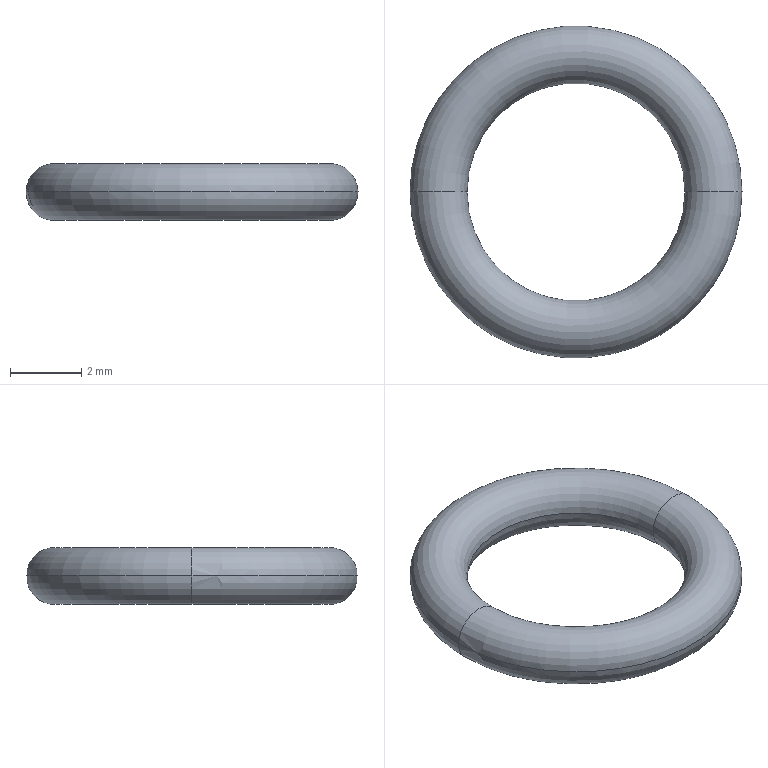Part | STEP file | o-rings_am_J515160x0061H | 1 solid | 4 faces | box 9.3 x 9.3 x 1.6 mm | volume 48.637 mm3 | torus 4
STEP:
#1=CARTESIAN_POINT('',(0.,0.,0.));
#2=DIRECTION('',(0.,0.,1.));
#3=DIRECTION('',(1.,0.,0.));
#4=AXIS2_PLACEMENT_3D('',#1,#2,#3);
#5=CARTESIAN_POINT('',(4.65,0.,0.));
#6=VERTEX_POINT('',#5);
#7=CARTESIAN_POINT('',(3.05,0.,0.));
#8=VERTEX_POINT('',#7);
#9=CARTESIAN_POINT('',(3.85,0.,0.));
#10=DIRECTION('',(0.,1.,0.));
#11=DIRECTION('',(-1.,0.,0.));
#12=AXIS2_PLACEMENT_3D('',#9,#10,#11);
#13=CIRCLE('',#12,0.8);
#14=CARTESIAN_POINT('',(0.,0.,0.));
#15=DIRECTION('',(0.,0.,-1.));
#16=DIRECTION('',(-1.,0.,0.));
#17=AXIS2_PLACEMENT_3D('',#14,#15,#16);
#18=TOROIDAL_SURFACE('',#17,3.85,0.8);
#19=CARTESIAN_POINT('',(3.142,-3.142));
#20=DIRECTION('',(0.,1.));
#21=VECTOR('',#20,1.);
#22=LINE('',#19,#21);
#23=(GEOMETRIC_REPRESENTATION_CONTEXT(2)PARAMETRIC_REPRESENTATION_CONTEXT()REPRESENTATION_CONTEXT('',''));
#24=DEFINITIONAL_REPRESENTATION('',(#22),#23);
#25=PCURVE('',#18,#24);
#26=CARTESIAN_POINT('',(0.,0.,0.));
#27=DIRECTION('',(0.,0.,-1.));
#28=DIRECTION('',(-1.,0.,0.));
#29=AXIS2_PLACEMENT_3D('',#26,#27,#28);
#30=TOROIDAL_SURFACE('',#29,3.85,0.8);
#31=CARTESIAN_POINT('',(3.142,-3.142));
#32=DIRECTION('',(0.,1.));
#33=VECTOR('',#32,1.);
#34=LINE('',#31,#33);
#35=(GEOMETRIC_REPRESENTATION_CONTEXT(2)PARAMETRIC_REPRESENTATION_CONTEXT()REPRESENTATION_CONTEXT('',''));
#36=DEFINITIONAL_REPRESENTATION('',(#34),#35);
#37=PCURVE('',#30,#36);
#38=SURFACE_CURVE('',#13,(#25,#37),.PCURVE_S1.);
#39=EDGE_CURVE('',#6,#8,#38,.T.);
#40=ORIENTED_EDGE('',*,*,#39,.F.);
#41=CARTESIAN_POINT('',(-4.65,0.,0.));
#42=VERTEX_POINT('',#41);
#43=CARTESIAN_POINT('',(0.,0.,0.));
#44=DIRECTION('',(0.,0.,-1.));
#45=DIRECTION('',(-1.,0.,0.));
#46=AXIS2_PLACEMENT_3D('',#43,#44,#45);
#47=CIRCLE('',#46,4.65);
#48=CARTESIAN_POINT('',(0.,0.));
#49=DIRECTION('',(1.,0.));
#50=VECTOR('',#49,1.);
#51=LINE('',#48,#50);
#52=(GEOMETRIC_REPRESENTATION_CONTEXT(2)PARAMETRIC_REPRESENTATION_CONTEXT()REPRESENTATION_CONTEXT('',''));
#53=DEFINITIONAL_REPRESENTATION('',(#51),#52);
#54=PCURVE('',#18,#53);
#55=CARTESIAN_POINT('',(0.,0.,0.));
#56=DIRECTION('',(0.,0.,-1.));
#57=DIRECTION('',(-1.,0.,0.));
#58=AXIS2_PLACEMENT_3D('',#55,#56,#57);
#59=TOROIDAL_SURFACE('',#58,3.85,0.8);
#60=CARTESIAN_POINT('',(0.,6.283));
#61=DIRECTION('',(1.,0.));
#62=VECTOR('',#61,1.);
#63=LINE('',#60,#62);
#64=(GEOMETRIC_REPRESENTATION_CONTEXT(2)PARAMETRIC_REPRESENTATION_CONTEXT()REPRESENTATION_CONTEXT('',''));
#65=DEFINITIONAL_REPRESENTATION('',(#63),#64);
#66=PCURVE('',#59,#65);
#67=SURFACE_CURVE('',#47,(#54,#66),.PCURVE_S1.);
#68=EDGE_CURVE('',#6,#42,#67,.T.);
#69=ORIENTED_EDGE('',*,*,#68,.T.);
#70=CARTESIAN_POINT('',(-3.05,0.,0.));
#71=VERTEX_POINT('',#70);
#72=CARTESIAN_POINT('',(-3.85,0.,0.));
#73=DIRECTION('',(0.,-1.,0.));
#74=DIRECTION('',(0.,0.,-1.));
#75=AXIS2_PLACEMENT_3D('',#72,#73,#74);
#76=CIRCLE('',#75,0.8);
#77=CARTESIAN_POINT('',(6.283,-4.712));
#78=DIRECTION('',(0.,1.));
#79=VECTOR('',#78,1.);
#80=LINE('',#77,#79);
#81=(GEOMETRIC_REPRESENTATION_CONTEXT(2)PARAMETRIC_REPRESENTATION_CONTEXT()REPRESENTATION_CONTEXT('',''));
#82=DEFINITIONAL_REPRESENTATION('',(#80),#81);
#83=PCURVE('',#18,#82);
#84=CARTESIAN_POINT('',(0.,-4.712));
#85=DIRECTION('',(0.,1.));
#86=VECTOR('',#85,1.);
#87=LINE('',#84,#86);
#88=(GEOMETRIC_REPRESENTATION_CONTEXT(2)PARAMETRIC_REPRESENTATION_CONTEXT()REPRESENTATION_CONTEXT('',''));
#89=DEFINITIONAL_REPRESENTATION('',(#87),#88);
#90=PCURVE('',#30,#89);
#91=SURFACE_CURVE('',#76,(#83,#90),.PCURVE_S1.);
#92=EDGE_CURVE('',#42,#71,#91,.T.);
#93=ORIENTED_EDGE('',*,*,#92,.T.);
#94=CARTESIAN_POINT('',(0.,0.,0.));
#95=DIRECTION('',(0.,0.,-1.));
#96=DIRECTION('',(-1.,0.,0.));
#97=AXIS2_PLACEMENT_3D('',#94,#95,#96);
#98=CIRCLE('',#97,3.05);
#99=CARTESIAN_POINT('',(0.,3.142));
#100=DIRECTION('',(1.,0.));
#101=VECTOR('',#100,1.);
#102=LINE('',#99,#101);
#103=(GEOMETRIC_REPRESENTATION_CONTEXT(2)PARAMETRIC_REPRESENTATION_CONTEXT()REPRESENTATION_CONTEXT('',''));
#104=DEFINITIONAL_REPRESENTATION('',(#102),#103);
#105=PCURVE('',#18,#104);
#106=CARTESIAN_POINT('',(0.,3.142));
#107=DIRECTION('',(1.,0.));
#108=VECTOR('',#107,1.);
#109=LINE('',#106,#108);
#110=(GEOMETRIC_REPRESENTATION_CONTEXT(2)PARAMETRIC_REPRESENTATION_CONTEXT()REPRESENTATION_CONTEXT('',''));
#111=DEFINITIONAL_REPRESENTATION('',(#109),#110);
#112=PCURVE('',#59,#111);
#113=SURFACE_CURVE('',#98,(#105,#112),.PCURVE_S1.);
#114=EDGE_CURVE('',#8,#71,#113,.T.);
#115=ORIENTED_EDGE('',*,*,#114,.F.);
#116=EDGE_LOOP('',(#40,#69,#93,#115));
#117=FACE_BOUND('',#116,.T.);
#118=ADVANCED_FACE('',(#117),#18,.T.);
#119=ORIENTED_EDGE('',*,*,#92,.F.);
#120=CARTESIAN_POINT('',(0.,0.,0.));
#121=DIRECTION('',(0.,0.,-1.));
#122=DIRECTION('',(-1.,0.,0.));
#123=AXIS2_PLACEMENT_3D('',#120,#121,#122);
#124=CIRCLE('',#123,4.65);
#125=CARTESIAN_POINT('',(0.,0.));
#126=DIRECTION('',(1.,0.));
#127=VECTOR('',#126,1.);
#128=LINE('',#125,#127);
#129=(GEOMETRIC_REPRESENTATION_CONTEXT(2)PARAMETRIC_REPRESENTATION_CONTEXT()REPRESENTATION_CONTEXT('',''));
#130=DEFINITIONAL_REPRESENTATION('',(#128),#129);
#131=PCURVE('',#30,#130);
#132=CARTESIAN_POINT('',(0.,0.,0.));
#133=DIRECTION('',(0.,0.,-1.));
#134=DIRECTION('',(-1.,0.,0.));
#135=AXIS2_PLACEMENT_3D('',#132,#133,#134);
#136=TOROIDAL_SURFACE('',#135,3.85,0.8);
#137=CARTESIAN_POINT('',(0.,6.283));
#138=DIRECTION('',(1.,0.));
#139=VECTOR('',#138,1.);
#140=LINE('',#137,#139);
#141=(GEOMETRIC_REPRESENTATION_CONTEXT(2)PARAMETRIC_REPRESENTATION_CONTEXT()REPRESENTATION_CONTEXT('',''));
#142=DEFINITIONAL_REPRESENTATION('',(#140),#141);
#143=PCURVE('',#136,#142);
#144=SURFACE_CURVE('',#124,(#131,#143),.PCURVE_S1.);
#145=EDGE_CURVE('',#42,#6,#144,.T.);
#146=ORIENTED_EDGE('',*,*,#145,.T.);
#147=ORIENTED_EDGE('',*,*,#39,.T.);
#148=CARTESIAN_POINT('',(0.,0.,0.));
#149=DIRECTION('',(0.,0.,-1.));
#150=DIRECTION('',(-1.,0.,0.));
#151=AXIS2_PLACEMENT_3D('',#148,#149,#150);
#152=CIRCLE('',#151,3.05);
#153=CARTESIAN_POINT('',(0.,3.142));
#154=DIRECTION('',(1.,0.));
#155=VECTOR('',#154,1.);
#156=LINE('',#153,#155);
#157=(GEOMETRIC_REPRESENTATION_CONTEXT(2)PARAMETRIC_REPRESENTATION_CONTEXT()REPRESENTATION_CONTEXT('',''));
#158=DEFINITIONAL_REPRESENTATION('',(#156),#157);
#159=PCURVE('',#30,#158);
#160=CARTESIAN_POINT('',(0.,3.142));
#161=DIRECTION('',(1.,0.));
#162=VECTOR('',#161,1.);
#163=LINE('',#160,#162);
#164=(GEOMETRIC_REPRESENTATION_CONTEXT(2)PARAMETRIC_REPRESENTATION_CONTEXT()REPRESENTATION_CONTEXT('',''));
#165=DEFINITIONAL_REPRESENTATION('',(#163),#164);
#166=PCURVE('',#136,#165);
#167=SURFACE_CURVE('',#152,(#159,#166),.PCURVE_S1.);
#168=EDGE_CURVE('',#71,#8,#167,.T.);
#169=ORIENTED_EDGE('',*,*,#168,.F.);
#170=EDGE_LOOP('',(#119,#146,#147,#169));
#171=FACE_BOUND('',#170,.T.);
#172=ADVANCED_FACE('',(#171),#30,.T.);
#173=ORIENTED_EDGE('',*,*,#145,.F.);
#174=CARTESIAN_POINT('',(-3.85,0.,0.));
#175=DIRECTION('',(0.,-1.,0.));
#176=DIRECTION('',(0.,0.,-1.));
#177=AXIS2_PLACEMENT_3D('',#174,#175,#176);
#178=CIRCLE('',#177,0.8);
#179=CARTESIAN_POINT('',(0.,1.571));
#180=DIRECTION('',(0.,1.));
#181=VECTOR('',#180,1.);
#182=LINE('',#179,#181);
#183=(GEOMETRIC_REPRESENTATION_CONTEXT(2)PARAMETRIC_REPRESENTATION_CONTEXT()REPRESENTATION_CONTEXT('',''));
#184=DEFINITIONAL_REPRESENTATION('',(#182),#183);
#185=PCURVE('',#136,#184);
#186=CARTESIAN_POINT('',(6.283,1.571));
#187=DIRECTION('',(0.,1.));
#188=VECTOR('',#187,1.);
#189=LINE('',#186,#188);
#190=(GEOMETRIC_REPRESENTATION_CONTEXT(2)PARAMETRIC_REPRESENTATION_CONTEXT()REPRESENTATION_CONTEXT('',''));
#191=DEFINITIONAL_REPRESENTATION('',(#189),#190);
#192=PCURVE('',#59,#191);
#193=SURFACE_CURVE('',#178,(#185,#192),.PCURVE_S1.);
#194=EDGE_CURVE('',#71,#42,#193,.T.);
#195=ORIENTED_EDGE('',*,*,#194,.F.);
#196=ORIENTED_EDGE('',*,*,#168,.T.);
#197=CARTESIAN_POINT('',(3.85,0.,0.));
#198=DIRECTION('',(0.,1.,0.));
#199=DIRECTION('',(-1.,0.,0.));
#200=AXIS2_PLACEMENT_3D('',#197,#198,#199);
#201=CIRCLE('',#200,0.8);
#202=CARTESIAN_POINT('',(3.142,3.142));
#203=DIRECTION('',(0.,1.));
#204=VECTOR('',#203,1.);
#205=LINE('',#202,#204);
#206=(GEOMETRIC_REPRESENTATION_CONTEXT(2)PARAMETRIC_REPRESENTATION_CONTEXT()REPRESENTATION_CONTEXT('',''));
#207=DEFINITIONAL_REPRESENTATION('',(#205),#206);
#208=PCURVE('',#136,#207);
#209=CARTESIAN_POINT('',(3.142,3.142));
#210=DIRECTION('',(0.,1.));
#211=VECTOR('',#210,1.);
#212=LINE('',#209,#211);
#213=(GEOMETRIC_REPRESENTATION_CONTEXT(2)PARAMETRIC_REPRESENTATION_CONTEXT()REPRESENTATION_CONTEXT('',''));
#214=DEFINITIONAL_REPRESENTATION('',(#212),#213);
#215=PCURVE('',#59,#214);
#216=SURFACE_CURVE('',#201,(#208,#215),.PCURVE_S1.);
#217=EDGE_CURVE('',#8,#6,#216,.T.);
#218=ORIENTED_EDGE('',*,*,#217,.T.);
#219=EDGE_LOOP('',(#173,#195,#196,#218));
#220=FACE_BOUND('',#219,.T.);
#221=ADVANCED_FACE('',(#220),#136,.T.);
#222=ORIENTED_EDGE('',*,*,#68,.F.);
#223=ORIENTED_EDGE('',*,*,#217,.F.);
#224=ORIENTED_EDGE('',*,*,#114,.T.);
#225=ORIENTED_EDGE('',*,*,#194,.T.);
#226=EDGE_LOOP('',(#222,#223,#224,#225));
#227=FACE_BOUND('',#226,.T.);
#228=ADVANCED_FACE('',(#227),#59,.T.);
#229=CLOSED_SHELL('',(#118,#172,#221,#228));
#230=MANIFOLD_SOLID_BREP('',#229);
#231=(LENGTH_UNIT()NAMED_UNIT(*)SI_UNIT(.MILLI.,.METRE.));
#232=UNCERTAINTY_MEASURE_WITH_UNIT(LENGTH_MEASURE(0.0000001),#231,'','');
#233=(NAMED_UNIT(*)PLANE_ANGLE_UNIT()SI_UNIT($,.RADIAN.));
#234=(NAMED_UNIT(*)SI_UNIT($,.STERADIAN.)SOLID_ANGLE_UNIT());
#235=(GEOMETRIC_REPRESENTATION_CONTEXT(3)GLOBAL_UNCERTAINTY_ASSIGNED_CONTEXT((#232))GLOBAL_UNIT_ASSIGNED_CONTEXT((#231,#233,#234))REPRESENTATION_CONTEXT('',''));
#236=ADVANCED_BREP_SHAPE_REPRESENTATION('',(#4,#230),#235);